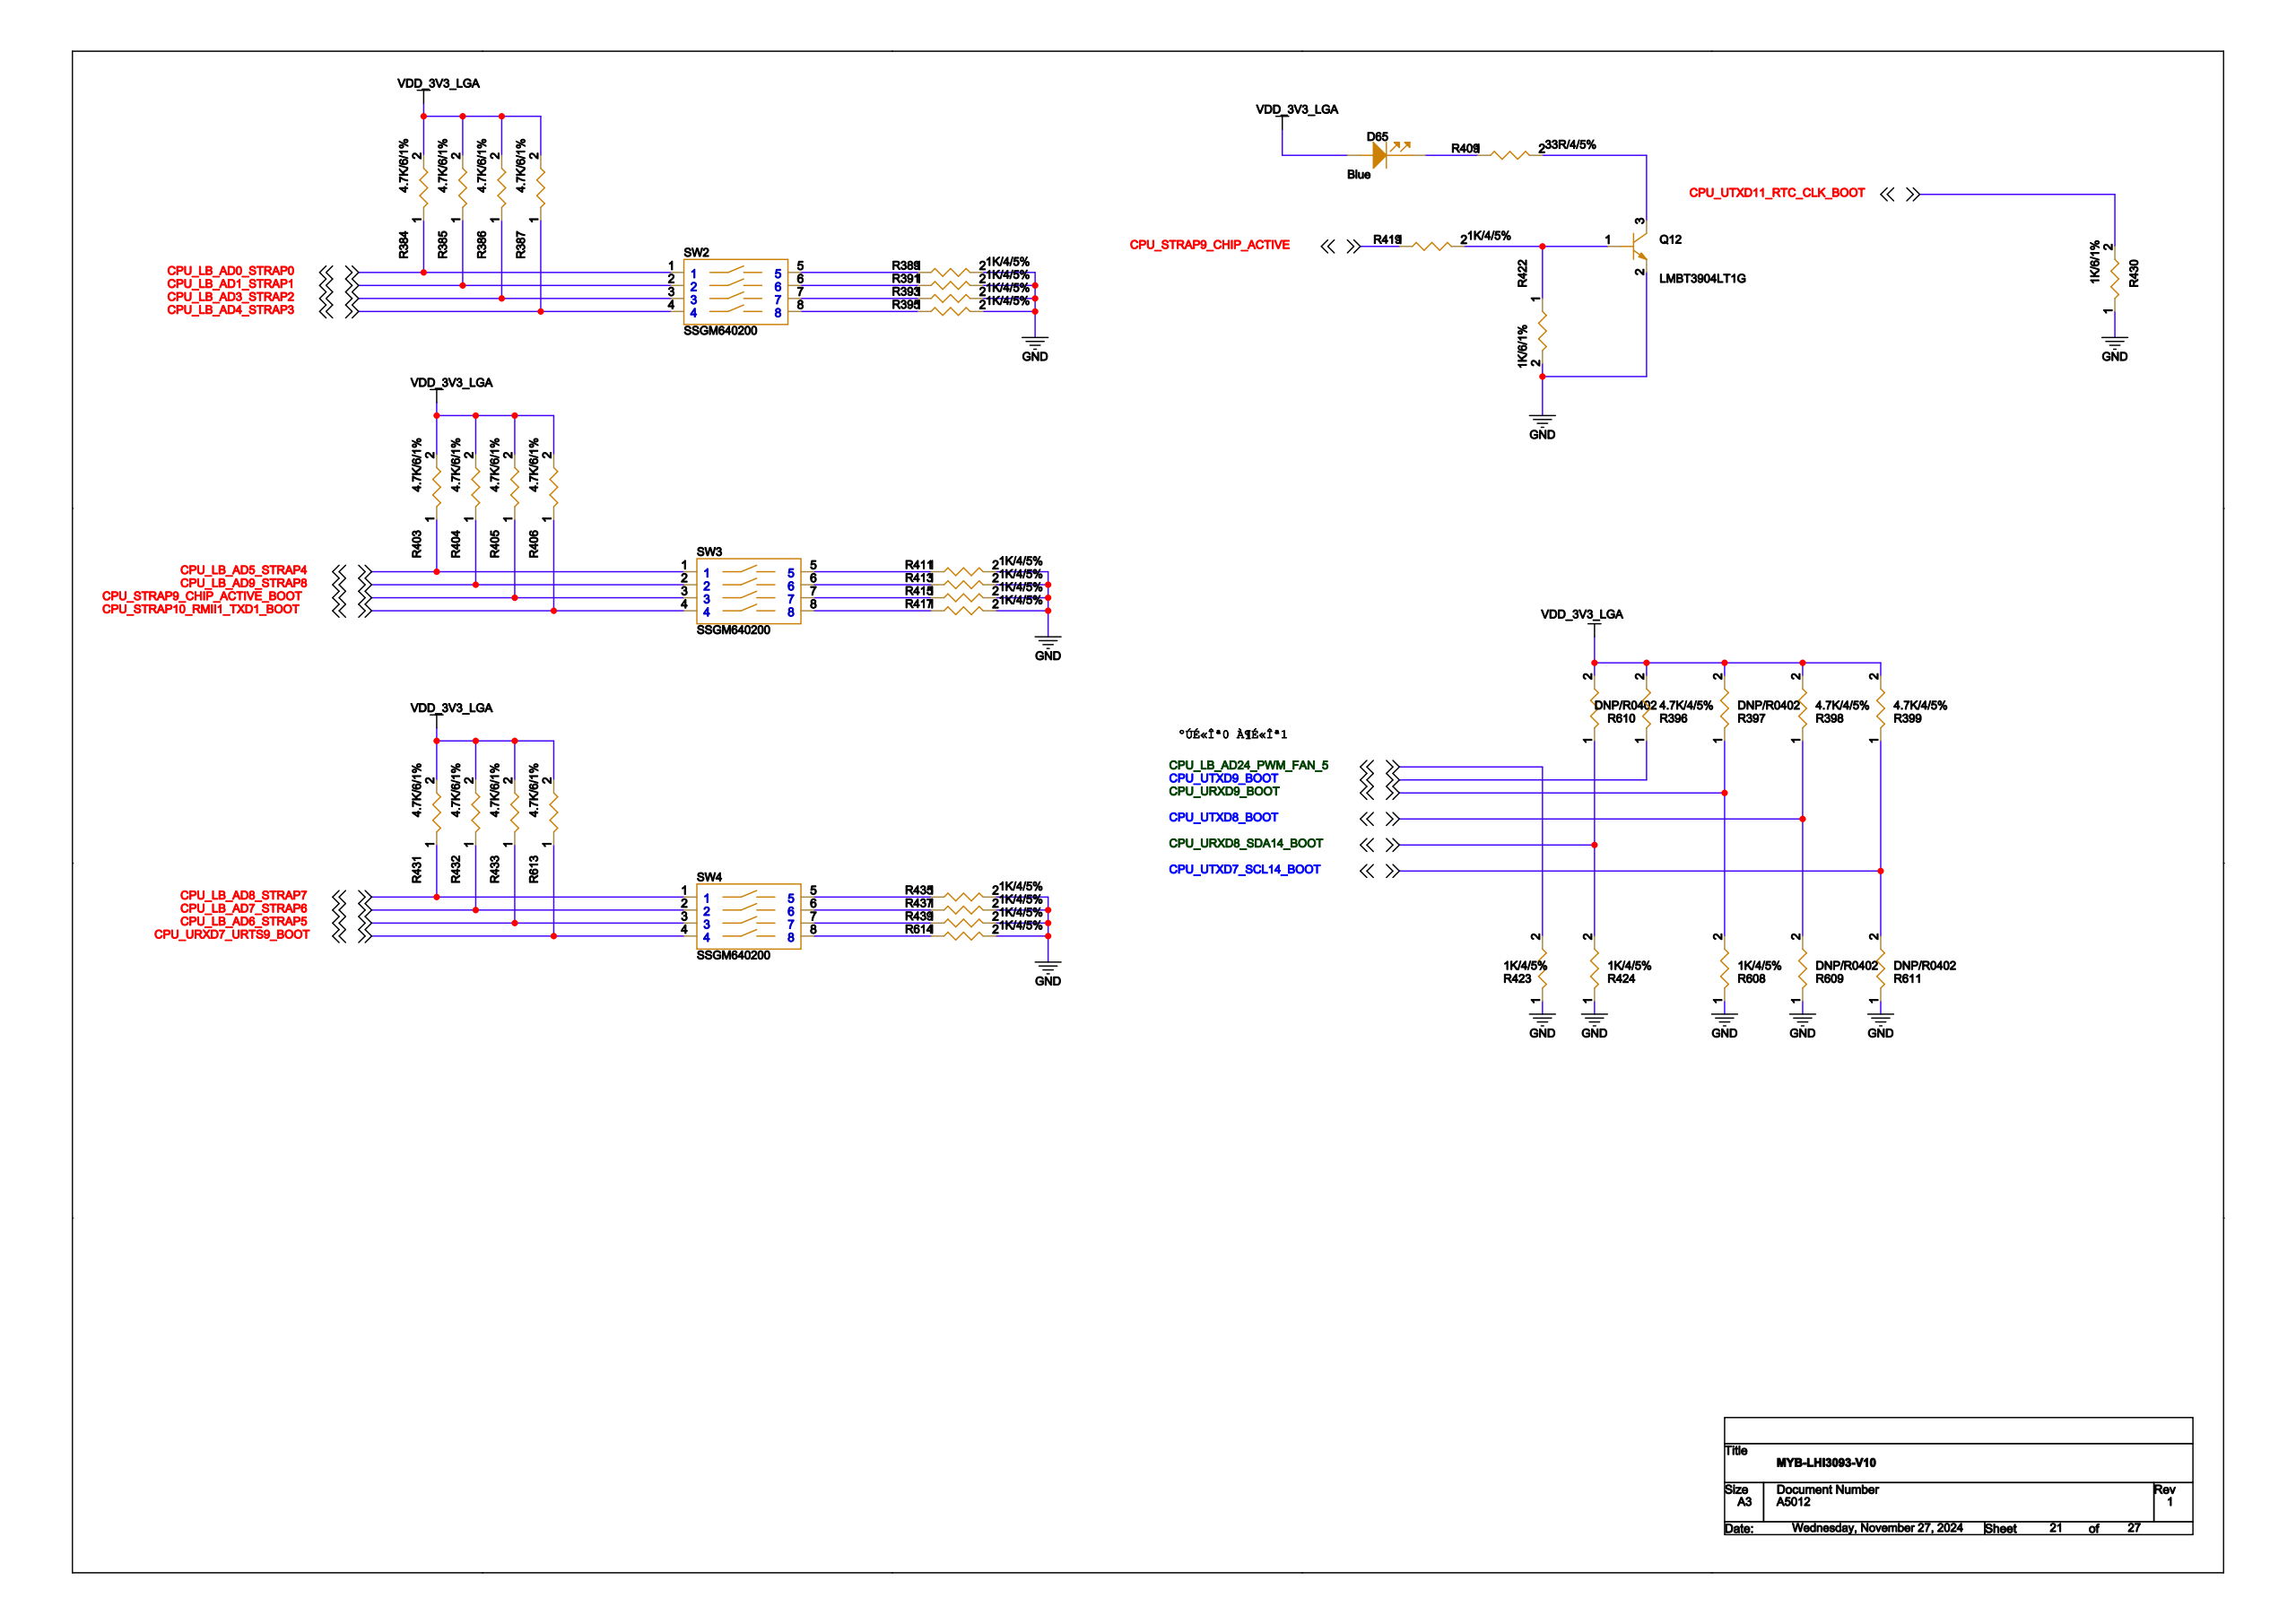Circuit board | Cadence Allegro | 1159 parts | 708 nets | one sheet of the schematic
Parts on this sheet (reference | value | footprint):
D65 | LED-SML1206 | LED0805
Q12 | LMBT3904LT1G | SOT-23
R384 | 4.7K/6/1% | R0402
R385 | 4.7K/6/1% | R0402
R386 | 4.7K/6/1% | R0402
R387 | 4.7K/6/1% | R0402
R396 | 4.7K/4/5% | R0402
R397 | DNP/R0402 | R0402
R398 | 4.7K/4/5% | R0402
R399 | 4.7K/4/5% | R0402
R403 | 4.7K/6/1% | R0402
R404 | 4.7K/6/1% | R0402
R405 | 4.7K/6/1% | R0402
R406 | 4.7K/6/1% | R0402
R422 | 1K/6/1% | R0402
R423 | 1K/4/5% | R0402
R424 | 1K/4/5% | R0402
R430 | 1K/6/1% | R0402
R431 | 4.7K/6/1% | R0402
R432 | 4.7K/6/1% | R0402
R433 | 4.7K/6/1% | R0402
R608 | 1K/4/5% | R0402
R609 | DNP/R0402 | R0402
R610 | DNP/R0402 | R0402
R611 | DNP/R0402 | R0402
R613 | 4.7K/6/1% | R0402
SW2 | SSGM640200 | SSGM640200
SW3 | SSGM640200 | SSGM640200
SW4 | SSGM640200 | SSGM640200
Nets of these parts (net: part-pin ...):
GND: Q12-2 R422-2 R423-1 R424-1 R430-1 R608-1 R609-1 R611-1
VDD_3V3_LGA: D65-1 R384-2 R385-2 R386-2 R387-2 R396-2 R397-2 R398-2 R399-2 R403-2 R404-2 R405-2 R406-2 R431-2 R432-2 R433-2 R610-2 R613-2
N15052802: D65-2
N15052806: Q12-3
N15052813: Q12-1 R422-1
N15049997: SW2-5
N15050001: SW2-6
N15050005: SW2-7
N15050009: SW2-8
N15050754: SW3-5
N15050758: SW3-6
N15050762: SW3-7
N15050766: SW3-8
CPU_LB_AD24_PWM_FAN_5: R423-2
CPU_URXD8_SDA14_BOOT: R424-2 R610-1
N15051494: SW4-5
N15051498: SW4-6
N15051502: SW4-7
CPU_LB_AD0_STRAP0: R384-1 SW2-1
CPU_LB_AD1_STRAP1: R385-1 SW2-2
CPU_LB_AD3_STRAP2: R386-1 SW2-3
CPU_LB_AD4_STRAP3: R387-1 SW2-4
CPU_LB_AD5_STRAP4: R403-1 SW3-1
CPU_LB_AD6_STRAP5: R433-1 SW4-3
CPU_LB_AD7_STRAP6: R432-1 SW4-2
CPU_LB_AD8_STRAP7: R431-1 SW4-1
CPU_LB_AD9_STRAP8: R404-1 SW3-2
CPU_URXD7_URTS9_BOOT: R613-1 SW4-4
CPU_UTXD7_SCL14_BOOT: R399-1 R611-2
CPU_UTXD11_RTC_CLK_BOOT: R430-2
CPU_UTXD8_BOOT: R398-1 R609-2
CPU_URXD9_BOOT: R397-1 R608-2
CPU_UTXD9_BOOT: R396-1
CPU_STRAP9_CHIP_ACTIVE_BOOT: R405-1 SW3-3
CPU_STRAP10_RMII1_TXD1_BOOT: R406-1 SW3-4
N15051506: SW4-8